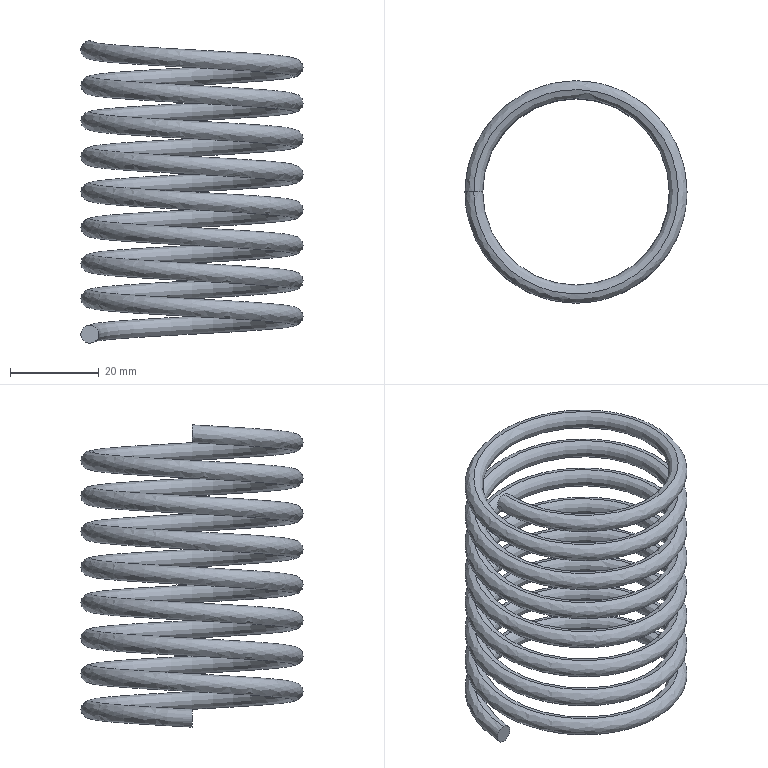Part | STEP file | helical spring | 1 solid | 4 faces | box 49.976 x 49.976 x 68 mm | volume 14534 mm3 | spline 2 | plane 2